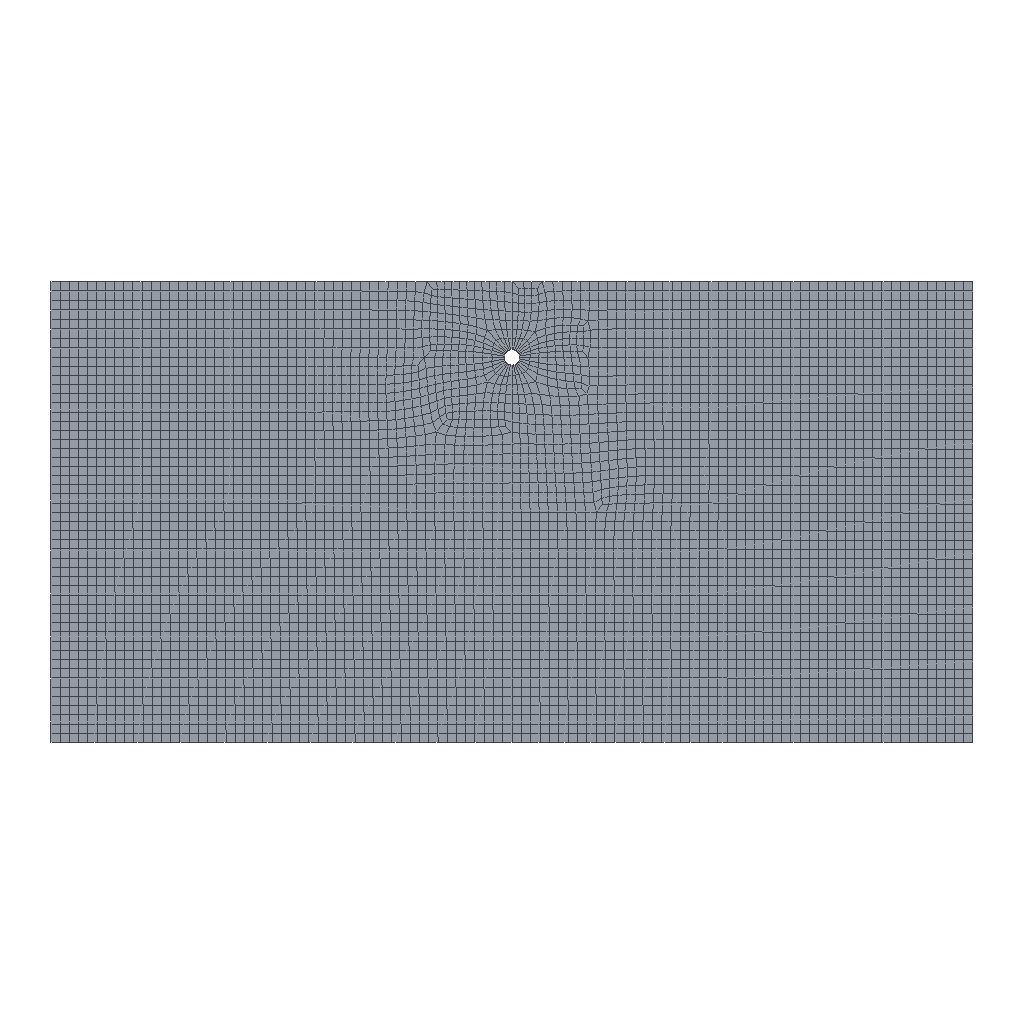Simulation study | abaqus
Set-up summary:
category,name,step,type,value,unit,region
solver,abaqus
solver,version,,,Abaqus/Standard 2020
solver,version,,,Abaqus/Standard 2020
units,not stated in the deck,,not stated
analysis,deck1,,soils,soils
load_step,Step-1,Step-1,soils,nlgeom=True
contact,interactions,,,general=0 pairs=0 ties=0
load_step,requested,,,1
mesh,nodes,,,5404
mesh,elements,,,5233
element_type,CPE4RP,,plane,5233
load,load commands in deck,,count,1
bc,support commands in deck,,count,4
analysis,deck2,,soils,soils
load_step,Step-1,Step-1,soils,nlgeom=True
contact,interactions,,,general=0 pairs=0 ties=0
load_step,requested,,,1
mesh,nodes,,,5404
mesh,elements,,,5233
element_type,CPE4RP,,plane,5233
load,load commands in deck,,count,1
bc,support commands in deck,,count,4
material,PIPE,,in results
material,SOIL,,in results
material,PIPE,,in results
material,SOIL,,in results
check,setup vs results,,match,"per instance, exact: element labels, types and connectivity; labels of the nodes the elements use; coordinates of those nodes at SINGLE_PRECISION in 1 of 1 instance(s)"
check,setup vs results,,match,"per instance, exact: element labels, types and connectivity; labels of the nodes the elements use; coordinates of those nodes at SINGLE_PRECISION in 1 of 1 instance(s)"
Results summary:
result,step,,completed,increments=17 time=100.0/100.0
result,analysis,,,soils
result,last_loadstep,,,1
result,analysis steps,,count,1
result,primary field,,,"U, POR"
result,reaction total,,FX,-3.8e-05,model units
result,reaction total,,FY,-1e-06,model units
result,reaction total,,FZ,0.0,model units
result,step,,completed,increments=17 time=100.0/100.0
result,analysis,,,soils
result,last_loadstep,,,1
result,analysis steps,,count,1
result,primary field,,,"U, POR"
result,reaction total,,FX,0.000244,model units
result,reaction total,,FY,-1.1e-05,model units
result,reaction total,,FZ,0.0,model units